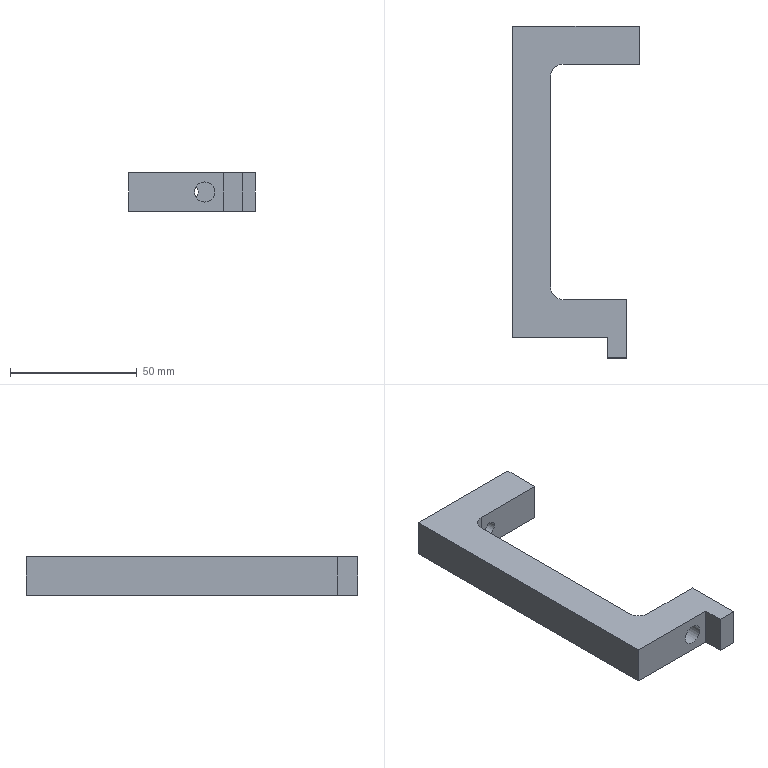Part | NX | features BREP 1 | 1 solid | 20 faces | box 50 x 131 x 15 mm | volume 41600 mm3 | plane 12 | cylinder 6 | cone 2 | commonest cylinder face diameters 6 x2 10 x2 5 x1 8 x1
STEP:
#1=CARTESIAN_POINT('',(30.,0.,11.5));
#2=VERTEX_POINT('',#1);
#3=CARTESIAN_POINT('',(30.,0.,7.5));
#4=DIRECTION('',(0.,1.,0.));
#5=DIRECTION('',(0.,0.,1.));
#6=AXIS2_PLACEMENT_3D('',#3,#4,#5);
#7=CIRCLE('',#6,4.);
#8=EDGE_CURVE('',#2,#2,#7,.T.);
#9=ORIENTED_EDGE('',*,*,#8,.T.);
#10=EDGE_LOOP('',(#9));
#11=FACE_BOUND('',#10,.T.);
#12=CARTESIAN_POINT('',(37.5,0.,15.));
#13=VERTEX_POINT('',#12);
#14=CARTESIAN_POINT('',(37.5,0.,0.));
#15=VERTEX_POINT('',#14);
#16=CARTESIAN_POINT('',(37.5,0.,15.));
#17=DIRECTION('',(0.,0.,-1.));
#18=VECTOR('',#17,1000.);
#19=LINE('',#16,#18);
#20=EDGE_CURVE('',#13,#15,#19,.T.);
#21=ORIENTED_EDGE('',*,*,#20,.F.);
#22=CARTESIAN_POINT('',(0.,0.,15.));
#23=VERTEX_POINT('',#22);
#24=CARTESIAN_POINT('',(0.,0.,15.));
#25=DIRECTION('',(1.,0.,0.));
#26=VECTOR('',#25,1000.);
#27=LINE('',#24,#26);
#28=EDGE_CURVE('',#23,#13,#27,.T.);
#29=ORIENTED_EDGE('',*,*,#28,.F.);
#30=CARTESIAN_POINT('',(0.,0.,0.));
#31=VERTEX_POINT('',#30);
#32=CARTESIAN_POINT('',(0.,0.,15.));
#33=DIRECTION('',(0.,0.,-1.));
#34=VECTOR('',#33,1000.);
#35=LINE('',#32,#34);
#36=EDGE_CURVE('',#23,#31,#35,.T.);
#37=ORIENTED_EDGE('',*,*,#36,.T.);
#38=CARTESIAN_POINT('',(0.,0.,0.));
#39=DIRECTION('',(1.,0.,0.));
#40=VECTOR('',#39,1000.);
#41=LINE('',#38,#40);
#42=EDGE_CURVE('',#31,#15,#41,.T.);
#43=ORIENTED_EDGE('',*,*,#42,.T.);
#44=EDGE_LOOP('',(#21,#29,#37,#43));
#45=FACE_BOUND('',#44,.T.);
#46=CARTESIAN_POINT('',(0.,0.,15.));
#47=DIRECTION('',(0.,1.,0.));
#48=DIRECTION('',(0.,0.,-1.));
#49=AXIS2_PLACEMENT_3D('',#46,#47,#48);
#50=PLANE('',#49);
#51=ADVANCED_FACE('',(#11,#45),#50,.F.);
#52=CARTESIAN_POINT('',(50.,108.,0.));
#53=VERTEX_POINT('',#52);
#54=CARTESIAN_POINT('',(50.,123.,0.));
#55=VERTEX_POINT('',#54);
#56=CARTESIAN_POINT('',(50.,108.,0.));
#57=DIRECTION('',(0.,1.,0.));
#58=VECTOR('',#57,1000.);
#59=LINE('',#56,#58);
#60=EDGE_CURVE('',#53,#55,#59,.T.);
#61=ORIENTED_EDGE('',*,*,#60,.T.);
#62=CARTESIAN_POINT('',(50.,123.,15.));
#63=VERTEX_POINT('',#62);
#64=CARTESIAN_POINT('',(50.,123.,15.));
#65=DIRECTION('',(0.,0.,-1.));
#66=VECTOR('',#65,1000.);
#67=LINE('',#64,#66);
#68=EDGE_CURVE('',#63,#55,#67,.T.);
#69=ORIENTED_EDGE('',*,*,#68,.F.);
#70=CARTESIAN_POINT('',(50.,108.,15.));
#71=VERTEX_POINT('',#70);
#72=CARTESIAN_POINT('',(50.,108.,15.));
#73=DIRECTION('',(0.,1.,0.));
#74=VECTOR('',#73,1000.);
#75=LINE('',#72,#74);
#76=EDGE_CURVE('',#71,#63,#75,.T.);
#77=ORIENTED_EDGE('',*,*,#76,.F.);
#78=CARTESIAN_POINT('',(50.,108.,15.));
#79=DIRECTION('',(0.,0.,-1.));
#80=VECTOR('',#79,1000.);
#81=LINE('',#78,#80);
#82=EDGE_CURVE('',#71,#53,#81,.T.);
#83=ORIENTED_EDGE('',*,*,#82,.T.);
#84=EDGE_LOOP('',(#61,#69,#77,#83));
#85=FACE_BOUND('',#84,.T.);
#86=CARTESIAN_POINT('',(50.,108.,15.));
#87=DIRECTION('',(-1.,0.,0.));
#88=DIRECTION('',(0.,1.,0.));
#89=AXIS2_PLACEMENT_3D('',#86,#87,#88);
#90=PLANE('',#89);
#91=ADVANCED_FACE('',(#85),#90,.F.);
#92=CARTESIAN_POINT('',(25.,123.,10.));
#93=VERTEX_POINT('',#92);
#94=CARTESIAN_POINT('',(25.,123.,7.5));
#95=DIRECTION('',(0.,1.,0.));
#96=DIRECTION('',(0.,0.,1.));
#97=AXIS2_PLACEMENT_3D('',#94,#95,#96);
#98=CIRCLE('',#97,2.5);
#99=EDGE_CURVE('',#93,#93,#98,.T.);
#100=ORIENTED_EDGE('',*,*,#99,.F.);
#101=EDGE_LOOP('',(#100));
#102=FACE_BOUND('',#101,.T.);
#103=CARTESIAN_POINT('',(43.,123.,10.5));
#104=VERTEX_POINT('',#103);
#105=CARTESIAN_POINT('',(43.,123.,7.5));
#106=DIRECTION('',(0.,1.,0.));
#107=DIRECTION('',(0.,0.,1.));
#108=AXIS2_PLACEMENT_3D('',#105,#106,#107);
#109=CIRCLE('',#108,3.);
#110=EDGE_CURVE('',#104,#104,#109,.T.);
#111=ORIENTED_EDGE('',*,*,#110,.F.);
#112=EDGE_LOOP('',(#111));
#113=FACE_BOUND('',#112,.T.);
#114=CARTESIAN_POINT('',(7.,123.,10.5));
#115=VERTEX_POINT('',#114);
#116=CARTESIAN_POINT('',(7.,123.,7.5));
#117=DIRECTION('',(0.,1.,0.));
#118=DIRECTION('',(0.,0.,1.));
#119=AXIS2_PLACEMENT_3D('',#116,#117,#118);
#120=CIRCLE('',#119,3.);
#121=EDGE_CURVE('',#115,#115,#120,.T.);
#122=ORIENTED_EDGE('',*,*,#121,.F.);
#123=EDGE_LOOP('',(#122));
#124=FACE_BOUND('',#123,.T.);
#125=CARTESIAN_POINT('',(0.,123.,0.));
#126=VERTEX_POINT('',#125);
#127=CARTESIAN_POINT('',(50.,123.,0.));
#128=DIRECTION('',(-1.,0.,0.));
#129=VECTOR('',#128,1000.);
#130=LINE('',#127,#129);
#131=EDGE_CURVE('',#55,#126,#130,.T.);
#132=ORIENTED_EDGE('',*,*,#131,.T.);
#133=CARTESIAN_POINT('',(0.,123.,15.));
#134=VERTEX_POINT('',#133);
#135=CARTESIAN_POINT('',(0.,123.,15.));
#136=DIRECTION('',(0.,0.,-1.));
#137=VECTOR('',#136,1000.);
#138=LINE('',#135,#137);
#139=EDGE_CURVE('',#134,#126,#138,.T.);
#140=ORIENTED_EDGE('',*,*,#139,.F.);
#141=CARTESIAN_POINT('',(50.,123.,15.));
#142=DIRECTION('',(-1.,0.,0.));
#143=VECTOR('',#142,1000.);
#144=LINE('',#141,#143);
#145=EDGE_CURVE('',#63,#134,#144,.T.);
#146=ORIENTED_EDGE('',*,*,#145,.F.);
#147=ORIENTED_EDGE('',*,*,#68,.T.);
#148=EDGE_LOOP('',(#132,#140,#146,#147));
#149=FACE_BOUND('',#148,.T.);
#150=CARTESIAN_POINT('',(50.,123.,15.));
#151=DIRECTION('',(0.,-1.,0.));
#152=DIRECTION('',(0.,0.,1.));
#153=AXIS2_PLACEMENT_3D('',#150,#151,#152);
#154=PLANE('',#153);
#155=ADVANCED_FACE('',(#102,#113,#124,#149),#154,.F.);
#156=CARTESIAN_POINT('',(0.,123.,0.));
#157=DIRECTION('',(0.,-1.,0.));
#158=VECTOR('',#157,1000.);
#159=LINE('',#156,#158);
#160=EDGE_CURVE('',#126,#31,#159,.T.);
#161=ORIENTED_EDGE('',*,*,#160,.T.);
#162=ORIENTED_EDGE('',*,*,#36,.F.);
#163=CARTESIAN_POINT('',(0.,123.,15.));
#164=DIRECTION('',(0.,-1.,0.));
#165=VECTOR('',#164,1000.);
#166=LINE('',#163,#165);
#167=EDGE_CURVE('',#134,#23,#166,.T.);
#168=ORIENTED_EDGE('',*,*,#167,.F.);
#169=ORIENTED_EDGE('',*,*,#139,.T.);
#170=EDGE_LOOP('',(#161,#162,#168,#169));
#171=FACE_BOUND('',#170,.T.);
#172=CARTESIAN_POINT('',(0.,123.,15.));
#173=DIRECTION('',(1.,0.,0.));
#174=DIRECTION('',(0.,-1.,0.));
#175=AXIS2_PLACEMENT_3D('',#172,#173,#174);
#176=PLANE('',#175);
#177=ADVANCED_FACE('',(#171),#176,.F.);
#178=CARTESIAN_POINT('',(45.,-8.,0.));
#179=VERTEX_POINT('',#178);
#180=CARTESIAN_POINT('',(45.,15.,0.));
#181=VERTEX_POINT('',#180);
#182=CARTESIAN_POINT('',(45.,0.,0.));
#183=DIRECTION('',(0.,1.,0.));
#184=VECTOR('',#183,1000.);
#185=LINE('',#182,#184);
#186=EDGE_CURVE('',#179,#181,#185,.T.);
#187=ORIENTED_EDGE('',*,*,#186,.T.);
#188=CARTESIAN_POINT('',(45.,15.,15.));
#189=VERTEX_POINT('',#188);
#190=CARTESIAN_POINT('',(45.,15.,15.));
#191=DIRECTION('',(0.,0.,-1.));
#192=VECTOR('',#191,1000.);
#193=LINE('',#190,#192);
#194=EDGE_CURVE('',#189,#181,#193,.T.);
#195=ORIENTED_EDGE('',*,*,#194,.F.);
#196=CARTESIAN_POINT('',(45.,-8.,15.));
#197=VERTEX_POINT('',#196);
#198=CARTESIAN_POINT('',(45.,0.,15.));
#199=DIRECTION('',(0.,1.,0.));
#200=VECTOR('',#199,1000.);
#201=LINE('',#198,#200);
#202=EDGE_CURVE('',#197,#189,#201,.T.);
#203=ORIENTED_EDGE('',*,*,#202,.F.);
#204=CARTESIAN_POINT('',(45.,-8.,15.));
#205=DIRECTION('',(0.,0.,-1.));
#206=VECTOR('',#205,1000.);
#207=LINE('',#204,#206);
#208=EDGE_CURVE('',#197,#179,#207,.T.);
#209=ORIENTED_EDGE('',*,*,#208,.T.);
#210=EDGE_LOOP('',(#187,#195,#203,#209));
#211=FACE_BOUND('',#210,.T.);
#212=CARTESIAN_POINT('',(45.,0.,15.));
#213=DIRECTION('',(-1.,0.,0.));
#214=DIRECTION('',(0.,0.,-1.));
#215=AXIS2_PLACEMENT_3D('',#212,#213,#214);
#216=PLANE('',#215);
#217=ADVANCED_FACE('',(#211),#216,.F.);
#218=CARTESIAN_POINT('',(30.,15.,11.5));
#219=VERTEX_POINT('',#218);
#220=CARTESIAN_POINT('',(30.,15.,7.5));
#221=DIRECTION('',(0.,1.,0.));
#222=DIRECTION('',(0.,0.,1.));
#223=AXIS2_PLACEMENT_3D('',#220,#221,#222);
#224=CIRCLE('',#223,4.);
#225=EDGE_CURVE('',#219,#219,#224,.T.);
#226=ORIENTED_EDGE('',*,*,#225,.F.);
#227=EDGE_LOOP('',(#226));
#228=FACE_BOUND('',#227,.T.);
#229=CARTESIAN_POINT('',(20.,15.,0.));
#230=VERTEX_POINT('',#229);
#231=CARTESIAN_POINT('',(45.,15.,0.));
#232=DIRECTION('',(-1.,0.,0.));
#233=VECTOR('',#232,1000.);
#234=LINE('',#231,#233);
#235=EDGE_CURVE('',#181,#230,#234,.T.);
#236=ORIENTED_EDGE('',*,*,#235,.T.);
#237=CARTESIAN_POINT('',(20.,15.,15.));
#238=VERTEX_POINT('',#237);
#239=CARTESIAN_POINT('',(20.,15.,15.));
#240=DIRECTION('',(0.,0.,1.));
#241=VECTOR('',#240,1000.);
#242=LINE('',#239,#241);
#243=EDGE_CURVE('',#230,#238,#242,.T.);
#244=ORIENTED_EDGE('',*,*,#243,.T.);
#245=CARTESIAN_POINT('',(45.,15.,15.));
#246=DIRECTION('',(-1.,0.,0.));
#247=VECTOR('',#246,1000.);
#248=LINE('',#245,#247);
#249=EDGE_CURVE('',#189,#238,#248,.T.);
#250=ORIENTED_EDGE('',*,*,#249,.F.);
#251=ORIENTED_EDGE('',*,*,#194,.T.);
#252=EDGE_LOOP('',(#236,#244,#250,#251));
#253=FACE_BOUND('',#252,.T.);
#254=CARTESIAN_POINT('',(45.,15.,15.));
#255=DIRECTION('',(0.,-1.,0.));
#256=DIRECTION('',(-1.,0.,0.));
#257=AXIS2_PLACEMENT_3D('',#254,#255,#256);
#258=PLANE('',#257);
#259=ADVANCED_FACE('',(#228,#253),#258,.F.);
#260=CARTESIAN_POINT('',(15.,20.,15.));
#261=VERTEX_POINT('',#260);
#262=CARTESIAN_POINT('',(15.,103.,15.));
#263=VERTEX_POINT('',#262);
#264=CARTESIAN_POINT('',(15.,15.,15.));
#265=DIRECTION('',(0.,1.,0.));
#266=VECTOR('',#265,1000.);
#267=LINE('',#264,#266);
#268=EDGE_CURVE('',#261,#263,#267,.T.);
#269=ORIENTED_EDGE('',*,*,#268,.F.);
#270=CARTESIAN_POINT('',(15.,20.,0.));
#271=VERTEX_POINT('',#270);
#272=CARTESIAN_POINT('',(15.,20.,0.));
#273=DIRECTION('',(0.,0.,-1.));
#274=VECTOR('',#273,1000.);
#275=LINE('',#272,#274);
#276=EDGE_CURVE('',#261,#271,#275,.T.);
#277=ORIENTED_EDGE('',*,*,#276,.T.);
#278=CARTESIAN_POINT('',(15.,103.,0.));
#279=VERTEX_POINT('',#278);
#280=CARTESIAN_POINT('',(15.,15.,0.));
#281=DIRECTION('',(0.,1.,0.));
#282=VECTOR('',#281,1000.);
#283=LINE('',#280,#282);
#284=EDGE_CURVE('',#271,#279,#283,.T.);
#285=ORIENTED_EDGE('',*,*,#284,.T.);
#286=CARTESIAN_POINT('',(15.,103.,15.));
#287=DIRECTION('',(0.,0.,1.));
#288=VECTOR('',#287,1000.);
#289=LINE('',#286,#288);
#290=EDGE_CURVE('',#279,#263,#289,.T.);
#291=ORIENTED_EDGE('',*,*,#290,.T.);
#292=EDGE_LOOP('',(#269,#277,#285,#291));
#293=FACE_BOUND('',#292,.T.);
#294=CARTESIAN_POINT('',(15.,15.,15.));
#295=DIRECTION('',(-1.,0.,0.));
#296=DIRECTION('',(0.,0.,-1.));
#297=AXIS2_PLACEMENT_3D('',#294,#295,#296);
#298=PLANE('',#297);
#299=ADVANCED_FACE('',(#293),#298,.F.);
#300=CARTESIAN_POINT('',(25.,108.,10.));
#301=VERTEX_POINT('',#300);
#302=CARTESIAN_POINT('',(25.,108.,7.5));
#303=DIRECTION('',(0.,1.,0.));
#304=DIRECTION('',(0.,0.,1.));
#305=AXIS2_PLACEMENT_3D('',#302,#303,#304);
#306=CIRCLE('',#305,2.5);
#307=EDGE_CURVE('',#301,#301,#306,.T.);
#308=ORIENTED_EDGE('',*,*,#307,.T.);
#309=EDGE_LOOP('',(#308));
#310=FACE_BOUND('',#309,.T.);
#311=CARTESIAN_POINT('',(20.,108.,15.));
#312=VERTEX_POINT('',#311);
#313=CARTESIAN_POINT('',(15.,108.,15.));
#314=DIRECTION('',(1.,0.,0.));
#315=VECTOR('',#314,1000.);
#316=LINE('',#313,#315);
#317=EDGE_CURVE('',#312,#71,#316,.T.);
#318=ORIENTED_EDGE('',*,*,#317,.F.);
#319=CARTESIAN_POINT('',(20.,108.,0.));
#320=VERTEX_POINT('',#319);
#321=CARTESIAN_POINT('',(20.,108.,0.));
#322=DIRECTION('',(0.,0.,-1.));
#323=VECTOR('',#322,1000.);
#324=LINE('',#321,#323);
#325=EDGE_CURVE('',#312,#320,#324,.T.);
#326=ORIENTED_EDGE('',*,*,#325,.T.);
#327=CARTESIAN_POINT('',(15.,108.,0.));
#328=DIRECTION('',(1.,0.,0.));
#329=VECTOR('',#328,1000.);
#330=LINE('',#327,#329);
#331=EDGE_CURVE('',#320,#53,#330,.T.);
#332=ORIENTED_EDGE('',*,*,#331,.T.);
#333=ORIENTED_EDGE('',*,*,#82,.F.);
#334=EDGE_LOOP('',(#318,#326,#332,#333));
#335=FACE_BOUND('',#334,.T.);
#336=CARTESIAN_POINT('',(15.,108.,15.));
#337=DIRECTION('',(0.,1.,0.));
#338=DIRECTION('',(0.,0.,-1.));
#339=AXIS2_PLACEMENT_3D('',#336,#337,#338);
#340=PLANE('',#339);
#341=ADVANCED_FACE('',(#310,#335),#340,.F.);
#342=ORIENTED_EDGE('',*,*,#76,.T.);
#343=ORIENTED_EDGE('',*,*,#145,.T.);
#344=ORIENTED_EDGE('',*,*,#167,.T.);
#345=ORIENTED_EDGE('',*,*,#28,.T.);
#346=CARTESIAN_POINT('',(37.5,-8.,15.));
#347=VERTEX_POINT('',#346);
#348=CARTESIAN_POINT('',(37.5,-8.,15.));
#349=DIRECTION('',(0.,1.,0.));
#350=VECTOR('',#349,1000.);
#351=LINE('',#348,#350);
#352=EDGE_CURVE('',#347,#13,#351,.T.);
#353=ORIENTED_EDGE('',*,*,#352,.F.);
#354=CARTESIAN_POINT('',(45.,-8.,15.));
#355=DIRECTION('',(-1.,0.,0.));
#356=VECTOR('',#355,1000.);
#357=LINE('',#354,#356);
#358=EDGE_CURVE('',#197,#347,#357,.T.);
#359=ORIENTED_EDGE('',*,*,#358,.F.);
#360=ORIENTED_EDGE('',*,*,#202,.T.);
#361=ORIENTED_EDGE('',*,*,#249,.T.);
#362=CARTESIAN_POINT('',(20.,20.,15.));
#363=DIRECTION('',(0.,0.,-1.));
#364=DIRECTION('',(1.,0.,0.));
#365=AXIS2_PLACEMENT_3D('',#362,#363,#364);
#366=CIRCLE('',#365,5.);
#367=EDGE_CURVE('',#238,#261,#366,.T.);
#368=ORIENTED_EDGE('',*,*,#367,.T.);
#369=ORIENTED_EDGE('',*,*,#268,.T.);
#370=CARTESIAN_POINT('',(20.,103.,15.));
#371=DIRECTION('',(0.,0.,-1.));
#372=DIRECTION('',(1.,0.,0.));
#373=AXIS2_PLACEMENT_3D('',#370,#371,#372);
#374=CIRCLE('',#373,5.);
#375=EDGE_CURVE('',#263,#312,#374,.T.);
#376=ORIENTED_EDGE('',*,*,#375,.T.);
#377=ORIENTED_EDGE('',*,*,#317,.T.);
#378=EDGE_LOOP('',(#342,#343,#344,#345,#353,#359,#360,#361,#368,#369,#376,#377));
#379=FACE_BOUND('',#378,.T.);
#380=CARTESIAN_POINT('',(0.,0.,15.));
#381=DIRECTION('',(0.,0.,1.));
#382=DIRECTION('',(-1.,0.,0.));
#383=AXIS2_PLACEMENT_3D('',#380,#381,#382);
#384=PLANE('',#383);
#385=ADVANCED_FACE('',(#379),#384,.T.);
#386=ORIENTED_EDGE('',*,*,#60,.F.);
#387=ORIENTED_EDGE('',*,*,#331,.F.);
#388=CARTESIAN_POINT('',(20.,103.,0.));
#389=DIRECTION('',(0.,0.,1.));
#390=DIRECTION('',(1.,0.,0.));
#391=AXIS2_PLACEMENT_3D('',#388,#389,#390);
#392=CIRCLE('',#391,5.);
#393=EDGE_CURVE('',#320,#279,#392,.T.);
#394=ORIENTED_EDGE('',*,*,#393,.T.);
#395=ORIENTED_EDGE('',*,*,#284,.F.);
#396=CARTESIAN_POINT('',(20.,20.,0.));
#397=DIRECTION('',(0.,0.,1.));
#398=DIRECTION('',(1.,0.,0.));
#399=AXIS2_PLACEMENT_3D('',#396,#397,#398);
#400=CIRCLE('',#399,5.);
#401=EDGE_CURVE('',#271,#230,#400,.T.);
#402=ORIENTED_EDGE('',*,*,#401,.T.);
#403=ORIENTED_EDGE('',*,*,#235,.F.);
#404=ORIENTED_EDGE('',*,*,#186,.F.);
#405=CARTESIAN_POINT('',(37.5,-8.,0.));
#406=VERTEX_POINT('',#405);
#407=CARTESIAN_POINT('',(45.,-8.,0.));
#408=DIRECTION('',(-1.,0.,0.));
#409=VECTOR('',#408,1000.);
#410=LINE('',#407,#409);
#411=EDGE_CURVE('',#179,#406,#410,.T.);
#412=ORIENTED_EDGE('',*,*,#411,.T.);
#413=CARTESIAN_POINT('',(37.5,-8.,0.));
#414=DIRECTION('',(0.,1.,0.));
#415=VECTOR('',#414,1000.);
#416=LINE('',#413,#415);
#417=EDGE_CURVE('',#406,#15,#416,.T.);
#418=ORIENTED_EDGE('',*,*,#417,.T.);
#419=ORIENTED_EDGE('',*,*,#42,.F.);
#420=ORIENTED_EDGE('',*,*,#160,.F.);
#421=ORIENTED_EDGE('',*,*,#131,.F.);
#422=EDGE_LOOP('',(#386,#387,#394,#395,#402,#403,#404,#412,#418,#419,#420,#421));
#423=FACE_BOUND('',#422,.T.);
#424=CARTESIAN_POINT('',(0.,0.,0.));
#425=DIRECTION('',(0.,0.,1.));
#426=DIRECTION('',(-1.,0.,0.));
#427=AXIS2_PLACEMENT_3D('',#424,#425,#426);
#428=PLANE('',#427);
#429=ADVANCED_FACE('',(#423),#428,.F.);
#430=ORIENTED_EDGE('',*,*,#367,.F.);
#431=ORIENTED_EDGE('',*,*,#243,.F.);
#432=ORIENTED_EDGE('',*,*,#401,.F.);
#433=ORIENTED_EDGE('',*,*,#276,.F.);
#434=EDGE_LOOP('',(#430,#431,#432,#433));
#435=FACE_BOUND('',#434,.T.);
#436=CARTESIAN_POINT('',(20.,20.,15.));
#437=DIRECTION('',(0.,0.,1.));
#438=DIRECTION('',(-1.,0.,0.));
#439=AXIS2_PLACEMENT_3D('',#436,#437,#438);
#440=CYLINDRICAL_SURFACE('',#439,5.);
#441=ADVANCED_FACE('',(#435),#440,.F.);
#442=ORIENTED_EDGE('',*,*,#375,.F.);
#443=ORIENTED_EDGE('',*,*,#290,.F.);
#444=ORIENTED_EDGE('',*,*,#393,.F.);
#445=ORIENTED_EDGE('',*,*,#325,.F.);
#446=EDGE_LOOP('',(#442,#443,#444,#445));
#447=FACE_BOUND('',#446,.T.);
#448=CARTESIAN_POINT('',(20.,103.,15.));
#449=DIRECTION('',(0.,0.,1.));
#450=DIRECTION('',(-1.,0.,0.));
#451=AXIS2_PLACEMENT_3D('',#448,#449,#450);
#452=CYLINDRICAL_SURFACE('',#451,5.);
#453=ADVANCED_FACE('',(#447),#452,.F.);
#454=ORIENTED_EDGE('',*,*,#417,.F.);
#455=CARTESIAN_POINT('',(37.5,-8.,15.));
#456=DIRECTION('',(0.,0.,-1.));
#457=VECTOR('',#456,1000.);
#458=LINE('',#455,#457);
#459=EDGE_CURVE('',#347,#406,#458,.T.);
#460=ORIENTED_EDGE('',*,*,#459,.F.);
#461=ORIENTED_EDGE('',*,*,#352,.T.);
#462=ORIENTED_EDGE('',*,*,#20,.T.);
#463=EDGE_LOOP('',(#454,#460,#461,#462));
#464=FACE_BOUND('',#463,.T.);
#465=CARTESIAN_POINT('',(37.5,-8.,15.));
#466=DIRECTION('',(-1.,0.,0.));
#467=DIRECTION('',(0.,0.,-1.));
#468=AXIS2_PLACEMENT_3D('',#465,#466,#467);
#469=PLANE('',#468);
#470=ADVANCED_FACE('',(#464),#469,.T.);
#471=ORIENTED_EDGE('',*,*,#411,.F.);
#472=ORIENTED_EDGE('',*,*,#208,.F.);
#473=ORIENTED_EDGE('',*,*,#358,.T.);
#474=ORIENTED_EDGE('',*,*,#459,.T.);
#475=EDGE_LOOP('',(#471,#472,#473,#474));
#476=FACE_BOUND('',#475,.T.);
#477=CARTESIAN_POINT('',(45.,-8.,15.));
#478=DIRECTION('',(0.,-1.,0.));
#479=DIRECTION('',(0.,0.,1.));
#480=AXIS2_PLACEMENT_3D('',#477,#478,#479);
#481=PLANE('',#480);
#482=ADVANCED_FACE('',(#476),#481,.T.);
#483=ORIENTED_EDGE('',*,*,#225,.T.);
#484=EDGE_LOOP('',(#483));
#485=FACE_BOUND('',#484,.T.);
#486=ORIENTED_EDGE('',*,*,#8,.F.);
#487=EDGE_LOOP('',(#486));
#488=FACE_BOUND('',#487,.T.);
#489=CARTESIAN_POINT('',(30.,15.,7.5));
#490=DIRECTION('',(0.,1.,0.));
#491=DIRECTION('',(0.,0.,-1.));
#492=AXIS2_PLACEMENT_3D('',#489,#490,#491);
#493=CYLINDRICAL_SURFACE('',#492,4.);
#494=ADVANCED_FACE('',(#485,#488),#493,.F.);
#495=CARTESIAN_POINT('',(7.,109.197,7.5));
#496=VERTEX_POINT('',#495);
#497=VERTEX_LOOP('',#496);
#498=FACE_BOUND('',#497,.T.);
#499=CARTESIAN_POINT('',(7.,111.,10.5));
#500=VERTEX_POINT('',#499);
#501=CARTESIAN_POINT('',(7.,111.,7.5));
#502=DIRECTION('',(0.,1.,0.));
#503=DIRECTION('',(0.,0.,1.));
#504=AXIS2_PLACEMENT_3D('',#501,#502,#503);
#505=CIRCLE('',#504,3.);
#506=EDGE_CURVE('',#500,#500,#505,.T.);
#507=ORIENTED_EDGE('',*,*,#506,.T.);
#508=EDGE_LOOP('',(#507));
#509=FACE_BOUND('',#508,.T.);
#510=CARTESIAN_POINT('',(7.,111.,7.5));
#511=DIRECTION('',(0.,1.,0.));
#512=DIRECTION('',(0.,0.,-1.));
#513=AXIS2_PLACEMENT_3D('',#510,#511,#512);
#514=CONICAL_SURFACE('',#513,3.,1.03);
#515=ADVANCED_FACE('',(#498,#509),#514,.F.);
#516=ORIENTED_EDGE('',*,*,#506,.F.);
#517=EDGE_LOOP('',(#516));
#518=FACE_BOUND('',#517,.T.);
#519=ORIENTED_EDGE('',*,*,#121,.T.);
#520=EDGE_LOOP('',(#519));
#521=FACE_BOUND('',#520,.T.);
#522=CARTESIAN_POINT('',(7.,123.,7.5));
#523=DIRECTION('',(0.,1.,0.));
#524=DIRECTION('',(0.,0.,-1.));
#525=AXIS2_PLACEMENT_3D('',#522,#523,#524);
#526=CYLINDRICAL_SURFACE('',#525,3.);
#527=ADVANCED_FACE('',(#518,#521),#526,.F.);
#528=CARTESIAN_POINT('',(43.,109.197,7.5));
#529=VERTEX_POINT('',#528);
#530=VERTEX_LOOP('',#529);
#531=FACE_BOUND('',#530,.T.);
#532=CARTESIAN_POINT('',(43.,111.,10.5));
#533=VERTEX_POINT('',#532);
#534=CARTESIAN_POINT('',(43.,111.,7.5));
#535=DIRECTION('',(0.,1.,0.));
#536=DIRECTION('',(0.,0.,1.));
#537=AXIS2_PLACEMENT_3D('',#534,#535,#536);
#538=CIRCLE('',#537,3.);
#539=EDGE_CURVE('',#533,#533,#538,.T.);
#540=ORIENTED_EDGE('',*,*,#539,.T.);
#541=EDGE_LOOP('',(#540));
#542=FACE_BOUND('',#541,.T.);
#543=CARTESIAN_POINT('',(43.,111.,7.5));
#544=DIRECTION('',(0.,1.,0.));
#545=DIRECTION('',(0.,0.,-1.));
#546=AXIS2_PLACEMENT_3D('',#543,#544,#545);
#547=CONICAL_SURFACE('',#546,3.,1.03);
#548=ADVANCED_FACE('',(#531,#542),#547,.F.);
#549=ORIENTED_EDGE('',*,*,#539,.F.);
#550=EDGE_LOOP('',(#549));
#551=FACE_BOUND('',#550,.T.);
#552=ORIENTED_EDGE('',*,*,#110,.T.);
#553=EDGE_LOOP('',(#552));
#554=FACE_BOUND('',#553,.T.);
#555=CARTESIAN_POINT('',(43.,123.,7.5));
#556=DIRECTION('',(0.,1.,0.));
#557=DIRECTION('',(0.,0.,-1.));
#558=AXIS2_PLACEMENT_3D('',#555,#556,#557);
#559=CYLINDRICAL_SURFACE('',#558,3.);
#560=ADVANCED_FACE('',(#551,#554),#559,.F.);
#561=ORIENTED_EDGE('',*,*,#307,.F.);
#562=EDGE_LOOP('',(#561));
#563=FACE_BOUND('',#562,.T.);
#564=ORIENTED_EDGE('',*,*,#99,.T.);
#565=EDGE_LOOP('',(#564));
#566=FACE_BOUND('',#565,.T.);
#567=CARTESIAN_POINT('',(25.,123.,7.5));
#568=DIRECTION('',(0.,1.,0.));
#569=DIRECTION('',(0.,0.,-1.));
#570=AXIS2_PLACEMENT_3D('',#567,#568,#569);
#571=CYLINDRICAL_SURFACE('',#570,2.5);
#572=ADVANCED_FACE('',(#563,#566),#571,.F.);
#573=CLOSED_SHELL('',(#51,#91,#155,#177,#217,#259,#299,#341,#385,#429,#441,#453,#470,#482,#494,#515,#527,#548,#560,#572));
#574=MANIFOLD_SOLID_BREP('',#573);
#575=(LENGTH_UNIT()NAMED_UNIT(*)SI_UNIT(.MILLI.,.METRE.));
#576=UNCERTAINTY_MEASURE_WITH_UNIT(LENGTH_MEASURE(0.00001),#575,'','');
#577=(NAMED_UNIT(*)PLANE_ANGLE_UNIT()SI_UNIT($,.RADIAN.));
#578=(NAMED_UNIT(*)SI_UNIT($,.STERADIAN.)SOLID_ANGLE_UNIT());
#579=(GEOMETRIC_REPRESENTATION_CONTEXT(3)GLOBAL_UNCERTAINTY_ASSIGNED_CONTEXT((#576))GLOBAL_UNIT_ASSIGNED_CONTEXT((#575,#577,#578))REPRESENTATION_CONTEXT('',''));
#580=ADVANCED_BREP_SHAPE_REPRESENTATION('',(#574),#579);